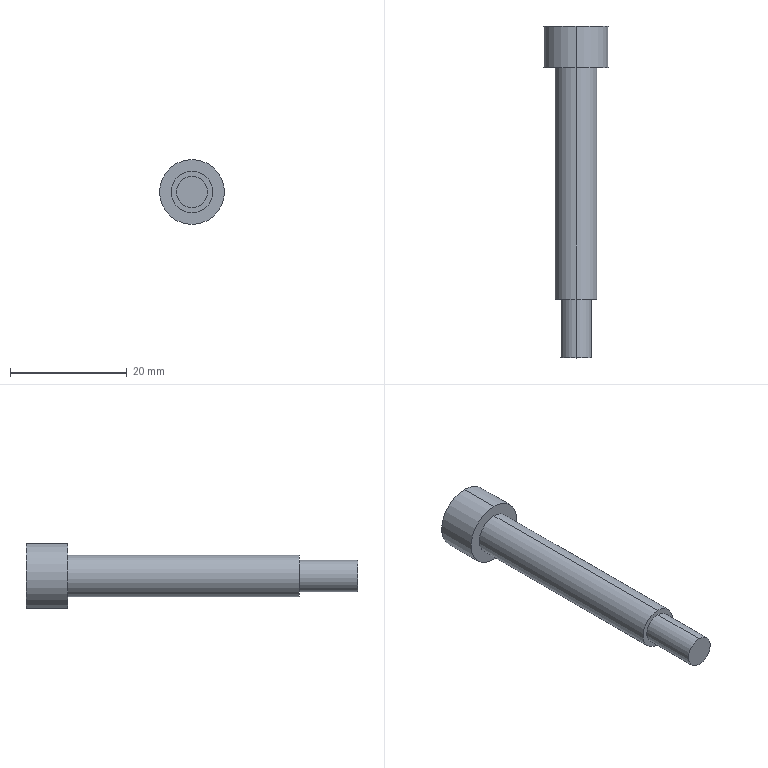Part | STEP file | 4-20.sldasm-Part-176 | 1 solid | 10 faces | box 11.113 x 56.8 x 11.112 mm | volume 2501 mm3 | cylinder 6 | plane 4 | commonest cylinder face diameters 5.319 x2 7.142 x2 11.112 x2
STEP:
#1=CARTESIAN_POINT('',(211.295,574.688,-128.256));
#2=VERTEX_POINT('',#1);
#3=CARTESIAN_POINT('',(211.295,574.688,-117.144));
#4=VERTEX_POINT('',#3);
#5=CARTESIAN_POINT('',(211.295,574.688,-122.7));
#6=DIRECTION('',(0.,1.,0.));
#7=DIRECTION('',(0.,0.,-1.));
#8=AXIS2_PLACEMENT_3D('',#5,#6,#7);
#9=CIRCLE('',#8,5.556);
#10=EDGE_CURVE('',#2,#4,#9,.T.);
#11=ORIENTED_EDGE('',*,*,#10,.T.);
#12=CARTESIAN_POINT('',(211.295,581.8,-117.144));
#13=VERTEX_POINT('',#12);
#14=CARTESIAN_POINT('',(211.295,574.688,-117.144));
#15=DIRECTION('',(0.,1.,0.));
#16=VECTOR('',#15,1000.);
#17=LINE('',#14,#16);
#18=EDGE_CURVE('',#4,#13,#17,.T.);
#19=ORIENTED_EDGE('',*,*,#18,.T.);
#20=CARTESIAN_POINT('',(211.295,581.8,-128.256));
#21=VERTEX_POINT('',#20);
#22=CARTESIAN_POINT('',(211.295,581.8,-122.7));
#23=DIRECTION('',(0.,1.,0.));
#24=DIRECTION('',(0.,0.,-1.));
#25=AXIS2_PLACEMENT_3D('',#22,#23,#24);
#26=CIRCLE('',#25,5.556);
#27=EDGE_CURVE('',#21,#13,#26,.T.);
#28=ORIENTED_EDGE('',*,*,#27,.F.);
#29=CARTESIAN_POINT('',(211.295,574.688,-128.256));
#30=DIRECTION('',(0.,1.,0.));
#31=VECTOR('',#30,1000.);
#32=LINE('',#29,#31);
#33=EDGE_CURVE('',#2,#21,#32,.T.);
#34=ORIENTED_EDGE('',*,*,#33,.F.);
#35=EDGE_LOOP('',(#11,#19,#28,#34));
#36=FACE_OUTER_BOUND('',#35,.T.);
#37=CARTESIAN_POINT('',(211.295,574.688,-122.7));
#38=DIRECTION('',(0.,1.,0.));
#39=DIRECTION('',(0.,0.,-1.));
#40=AXIS2_PLACEMENT_3D('',#37,#38,#39);
#41=CYLINDRICAL_SURFACE('',#40,5.556);
#42=ADVANCED_FACE('',(#36),#41,.T.);
#43=CARTESIAN_POINT('',(211.295,574.688,-119.129));
#44=VERTEX_POINT('',#43);
#45=CARTESIAN_POINT('',(211.295,574.688,-126.271));
#46=VERTEX_POINT('',#45);
#47=CARTESIAN_POINT('',(211.295,574.688,-122.7));
#48=DIRECTION('',(0.,-1.,0.));
#49=DIRECTION('',(0.,0.,1.));
#50=AXIS2_PLACEMENT_3D('',#47,#48,#49);
#51=CIRCLE('',#50,3.571);
#52=EDGE_CURVE('',#44,#46,#51,.T.);
#53=ORIENTED_EDGE('',*,*,#52,.T.);
#54=CARTESIAN_POINT('',(211.295,535.064,-126.271));
#55=VERTEX_POINT('',#54);
#56=CARTESIAN_POINT('',(211.295,574.688,-126.271));
#57=DIRECTION('',(0.,-1.,0.));
#58=VECTOR('',#57,1000.);
#59=LINE('',#56,#58);
#60=EDGE_CURVE('',#46,#55,#59,.T.);
#61=ORIENTED_EDGE('',*,*,#60,.T.);
#62=CARTESIAN_POINT('',(211.295,535.064,-119.129));
#63=VERTEX_POINT('',#62);
#64=CARTESIAN_POINT('',(211.295,535.064,-122.7));
#65=DIRECTION('',(0.,-1.,0.));
#66=DIRECTION('',(0.,0.,1.));
#67=AXIS2_PLACEMENT_3D('',#64,#65,#66);
#68=CIRCLE('',#67,3.571);
#69=EDGE_CURVE('',#63,#55,#68,.T.);
#70=ORIENTED_EDGE('',*,*,#69,.F.);
#71=CARTESIAN_POINT('',(211.295,574.688,-119.129));
#72=DIRECTION('',(0.,-1.,0.));
#73=VECTOR('',#72,1000.);
#74=LINE('',#71,#73);
#75=EDGE_CURVE('',#44,#63,#74,.T.);
#76=ORIENTED_EDGE('',*,*,#75,.F.);
#77=EDGE_LOOP('',(#53,#61,#70,#76));
#78=FACE_OUTER_BOUND('',#77,.T.);
#79=CARTESIAN_POINT('',(211.295,574.688,-122.7));
#80=DIRECTION('',(0.,-1.,0.));
#81=DIRECTION('',(0.,0.,1.));
#82=AXIS2_PLACEMENT_3D('',#79,#80,#81);
#83=CYLINDRICAL_SURFACE('',#82,3.571);
#84=ADVANCED_FACE('',(#78),#83,.T.);
#85=CARTESIAN_POINT('',(211.295,535.064,-120.041));
#86=VERTEX_POINT('',#85);
#87=CARTESIAN_POINT('',(211.295,535.064,-125.359));
#88=VERTEX_POINT('',#87);
#89=CARTESIAN_POINT('',(211.295,535.064,-122.7));
#90=DIRECTION('',(0.,-1.,0.));
#91=DIRECTION('',(0.,0.,1.));
#92=AXIS2_PLACEMENT_3D('',#89,#90,#91);
#93=CIRCLE('',#92,2.659);
#94=EDGE_CURVE('',#86,#88,#93,.T.);
#95=ORIENTED_EDGE('',*,*,#94,.T.);
#96=CARTESIAN_POINT('',(211.295,525.,-125.359));
#97=VERTEX_POINT('',#96);
#98=CARTESIAN_POINT('',(211.295,574.688,-125.359));
#99=DIRECTION('',(0.,-1.,0.));
#100=VECTOR('',#99,1000.);
#101=LINE('',#98,#100);
#102=EDGE_CURVE('',#88,#97,#101,.T.);
#103=ORIENTED_EDGE('',*,*,#102,.T.);
#104=CARTESIAN_POINT('',(211.295,525.,-120.041));
#105=VERTEX_POINT('',#104);
#106=CARTESIAN_POINT('',(211.295,525.,-122.7));
#107=DIRECTION('',(0.,-1.,0.));
#108=DIRECTION('',(0.,0.,1.));
#109=AXIS2_PLACEMENT_3D('',#106,#107,#108);
#110=CIRCLE('',#109,2.659);
#111=EDGE_CURVE('',#105,#97,#110,.T.);
#112=ORIENTED_EDGE('',*,*,#111,.F.);
#113=CARTESIAN_POINT('',(211.295,574.688,-120.041));
#114=DIRECTION('',(0.,-1.,0.));
#115=VECTOR('',#114,1000.);
#116=LINE('',#113,#115);
#117=EDGE_CURVE('',#86,#105,#116,.T.);
#118=ORIENTED_EDGE('',*,*,#117,.F.);
#119=EDGE_LOOP('',(#95,#103,#112,#118));
#120=FACE_OUTER_BOUND('',#119,.T.);
#121=CARTESIAN_POINT('',(211.295,574.688,-122.7));
#122=DIRECTION('',(0.,-1.,0.));
#123=DIRECTION('',(0.,0.,1.));
#124=AXIS2_PLACEMENT_3D('',#121,#122,#123);
#125=CYLINDRICAL_SURFACE('',#124,2.659);
#126=ADVANCED_FACE('',(#120),#125,.T.);
#127=ORIENTED_EDGE('',*,*,#102,.F.);
#128=CARTESIAN_POINT('',(211.295,535.064,-122.7));
#129=DIRECTION('',(0.,-1.,0.));
#130=DIRECTION('',(0.,0.,1.));
#131=AXIS2_PLACEMENT_3D('',#128,#129,#130);
#132=CIRCLE('',#131,2.659);
#133=EDGE_CURVE('',#88,#86,#132,.T.);
#134=ORIENTED_EDGE('',*,*,#133,.T.);
#135=ORIENTED_EDGE('',*,*,#117,.T.);
#136=CARTESIAN_POINT('',(211.295,525.,-122.7));
#137=DIRECTION('',(0.,-1.,0.));
#138=DIRECTION('',(0.,0.,1.));
#139=AXIS2_PLACEMENT_3D('',#136,#137,#138);
#140=CIRCLE('',#139,2.659);
#141=EDGE_CURVE('',#97,#105,#140,.T.);
#142=ORIENTED_EDGE('',*,*,#141,.F.);
#143=EDGE_LOOP('',(#127,#134,#135,#142));
#144=FACE_OUTER_BOUND('',#143,.T.);
#145=CARTESIAN_POINT('',(211.295,574.688,-122.7));
#146=DIRECTION('',(0.,-1.,0.));
#147=DIRECTION('',(0.,0.,1.));
#148=AXIS2_PLACEMENT_3D('',#145,#146,#147);
#149=CYLINDRICAL_SURFACE('',#148,2.659);
#150=ADVANCED_FACE('',(#144),#149,.T.);
#151=ORIENTED_EDGE('',*,*,#69,.T.);
#152=CARTESIAN_POINT('',(211.295,535.064,-122.7));
#153=DIRECTION('',(0.,-1.,0.));
#154=DIRECTION('',(0.,0.,1.));
#155=AXIS2_PLACEMENT_3D('',#152,#153,#154);
#156=CIRCLE('',#155,3.571);
#157=EDGE_CURVE('',#55,#63,#156,.T.);
#158=ORIENTED_EDGE('',*,*,#157,.T.);
#159=EDGE_LOOP('',(#151,#158));
#160=FACE_OUTER_BOUND('',#159,.T.);
#161=ORIENTED_EDGE('',*,*,#94,.F.);
#162=ORIENTED_EDGE('',*,*,#133,.F.);
#163=EDGE_LOOP('',(#161,#162));
#164=FACE_BOUND('',#163,.T.);
#165=CARTESIAN_POINT('',(211.295,535.064,-122.7));
#166=DIRECTION('',(0.,-1.,0.));
#167=DIRECTION('',(0.,0.,1.));
#168=AXIS2_PLACEMENT_3D('',#165,#166,#167);
#169=PLANE('',#168);
#170=ADVANCED_FACE('',(#160,#164),#169,.T.);
#171=ORIENTED_EDGE('',*,*,#60,.F.);
#172=CARTESIAN_POINT('',(211.295,574.688,-122.7));
#173=DIRECTION('',(0.,-1.,0.));
#174=DIRECTION('',(0.,0.,1.));
#175=AXIS2_PLACEMENT_3D('',#172,#173,#174);
#176=CIRCLE('',#175,3.571);
#177=EDGE_CURVE('',#46,#44,#176,.T.);
#178=ORIENTED_EDGE('',*,*,#177,.T.);
#179=ORIENTED_EDGE('',*,*,#75,.T.);
#180=ORIENTED_EDGE('',*,*,#157,.F.);
#181=EDGE_LOOP('',(#171,#178,#179,#180));
#182=FACE_OUTER_BOUND('',#181,.T.);
#183=CARTESIAN_POINT('',(211.295,574.688,-122.7));
#184=DIRECTION('',(0.,-1.,0.));
#185=DIRECTION('',(0.,0.,1.));
#186=AXIS2_PLACEMENT_3D('',#183,#184,#185);
#187=CYLINDRICAL_SURFACE('',#186,3.571);
#188=ADVANCED_FACE('',(#182),#187,.T.);
#189=ORIENTED_EDGE('',*,*,#27,.T.);
#190=CARTESIAN_POINT('',(211.295,581.8,-122.7));
#191=DIRECTION('',(0.,1.,0.));
#192=DIRECTION('',(0.,0.,-1.));
#193=AXIS2_PLACEMENT_3D('',#190,#191,#192);
#194=CIRCLE('',#193,5.556);
#195=EDGE_CURVE('',#13,#21,#194,.T.);
#196=ORIENTED_EDGE('',*,*,#195,.T.);
#197=EDGE_LOOP('',(#189,#196));
#198=FACE_OUTER_BOUND('',#197,.T.);
#199=CARTESIAN_POINT('',(211.295,581.8,-122.7));
#200=DIRECTION('',(0.,1.,0.));
#201=DIRECTION('',(0.,0.,-1.));
#202=AXIS2_PLACEMENT_3D('',#199,#200,#201);
#203=PLANE('',#202);
#204=ADVANCED_FACE('',(#198),#203,.T.);
#205=ORIENTED_EDGE('',*,*,#18,.F.);
#206=CARTESIAN_POINT('',(211.295,574.688,-122.7));
#207=DIRECTION('',(0.,1.,0.));
#208=DIRECTION('',(0.,0.,-1.));
#209=AXIS2_PLACEMENT_3D('',#206,#207,#208);
#210=CIRCLE('',#209,5.556);
#211=EDGE_CURVE('',#4,#2,#210,.T.);
#212=ORIENTED_EDGE('',*,*,#211,.T.);
#213=ORIENTED_EDGE('',*,*,#33,.T.);
#214=ORIENTED_EDGE('',*,*,#195,.F.);
#215=EDGE_LOOP('',(#205,#212,#213,#214));
#216=FACE_OUTER_BOUND('',#215,.T.);
#217=CARTESIAN_POINT('',(211.295,574.688,-122.7));
#218=DIRECTION('',(0.,1.,0.));
#219=DIRECTION('',(0.,0.,-1.));
#220=AXIS2_PLACEMENT_3D('',#217,#218,#219);
#221=CYLINDRICAL_SURFACE('',#220,5.556);
#222=ADVANCED_FACE('',(#216),#221,.T.);
#223=ORIENTED_EDGE('',*,*,#52,.F.);
#224=ORIENTED_EDGE('',*,*,#177,.F.);
#225=EDGE_LOOP('',(#223,#224));
#226=FACE_BOUND('',#225,.T.);
#227=ORIENTED_EDGE('',*,*,#10,.F.);
#228=ORIENTED_EDGE('',*,*,#211,.F.);
#229=EDGE_LOOP('',(#227,#228));
#230=FACE_OUTER_BOUND('',#229,.T.);
#231=CARTESIAN_POINT('',(211.295,574.688,-122.7));
#232=DIRECTION('',(0.,-1.,0.));
#233=DIRECTION('',(0.,0.,1.));
#234=AXIS2_PLACEMENT_3D('',#231,#232,#233);
#235=PLANE('',#234);
#236=ADVANCED_FACE('',(#226,#230),#235,.T.);
#237=ORIENTED_EDGE('',*,*,#111,.T.);
#238=ORIENTED_EDGE('',*,*,#141,.T.);
#239=EDGE_LOOP('',(#237,#238));
#240=FACE_OUTER_BOUND('',#239,.T.);
#241=CARTESIAN_POINT('',(263.495,525.,-98.65));
#242=DIRECTION('',(0.,-1.,0.));
#243=DIRECTION('',(0.,0.,1.));
#244=AXIS2_PLACEMENT_3D('',#241,#242,#243);
#245=PLANE('',#244);
#246=ADVANCED_FACE('',(#240),#245,.T.);
#247=CLOSED_SHELL('',(#42,#84,#126,#150,#170,#188,#204,#222,#236,#246));
#248=MANIFOLD_SOLID_BREP('',#247);
#249=CARTESIAN_POINT('',(0.,0.,0.));
#250=DIRECTION('',(0.,0.,1.));
#251=DIRECTION('',(1.,0.,0.));
#252=AXIS2_PLACEMENT_3D('',#249,#250,#251);
#253=(LENGTH_UNIT()NAMED_UNIT(*)SI_UNIT(.MILLI.,.METRE.));
#254=UNCERTAINTY_MEASURE_WITH_UNIT(LENGTH_MEASURE(0.00001),#253,'','');
#255=(NAMED_UNIT(*)PLANE_ANGLE_UNIT()SI_UNIT($,.RADIAN.));
#256=(NAMED_UNIT(*)SI_UNIT($,.STERADIAN.)SOLID_ANGLE_UNIT());
#257=(GEOMETRIC_REPRESENTATION_CONTEXT(3)GLOBAL_UNCERTAINTY_ASSIGNED_CONTEXT((#254))GLOBAL_UNIT_ASSIGNED_CONTEXT((#253,#255,#256))REPRESENTATION_CONTEXT('',''));
#258=ADVANCED_BREP_SHAPE_REPRESENTATION('',(#248,#252),#257);